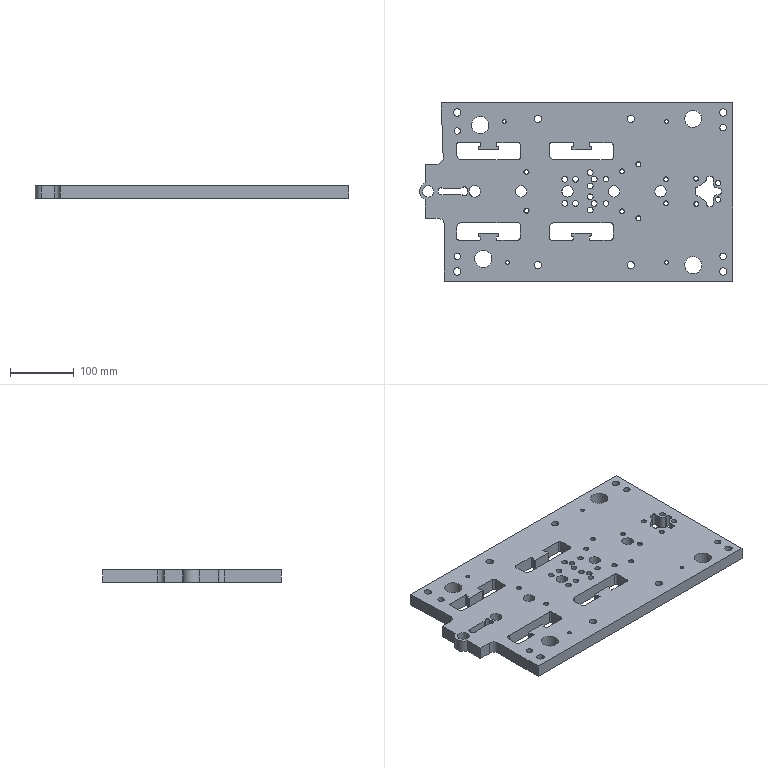Part | NX | features LB-17 2 | 1 solid | 223 faces | box 492.396 x 280 x 20 mm | volume 2253052 mm3 | cylinder 122 | plane 82 | cone 16 | spline 3 | commonest cylinder face diameters 1.76 x16 6 x12 2 x8 2.24 x8 6.8 x8 7.24 x8